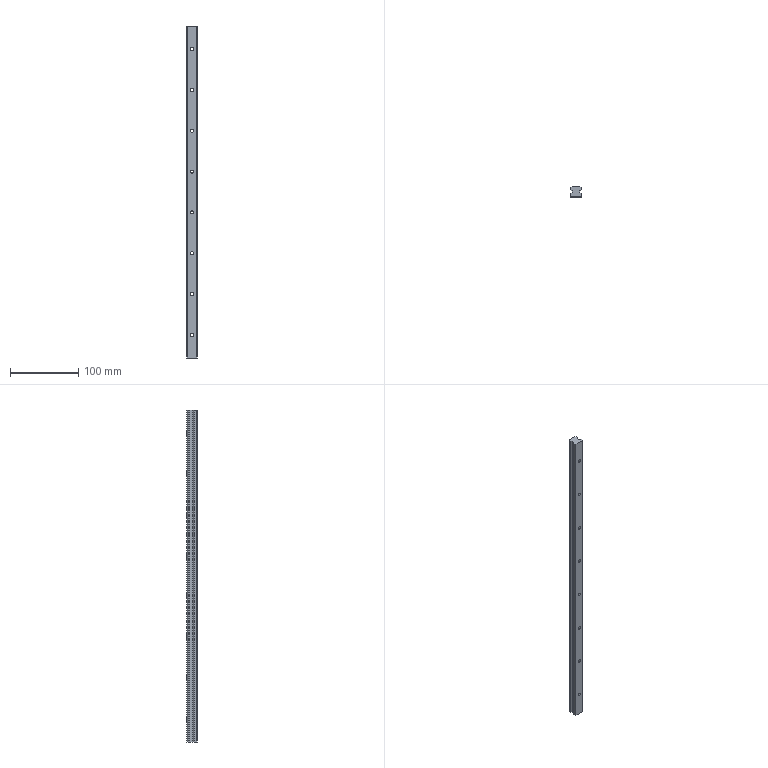Part | SolidWorks | features BaseBody 1 | 1 solid | 58 faces | box 15 x 15 x 488 mm | volume 95639 mm3 | cylinder 32 | plane 26 | commonest cylinder face diameters 4.5 x16 7.5 x16